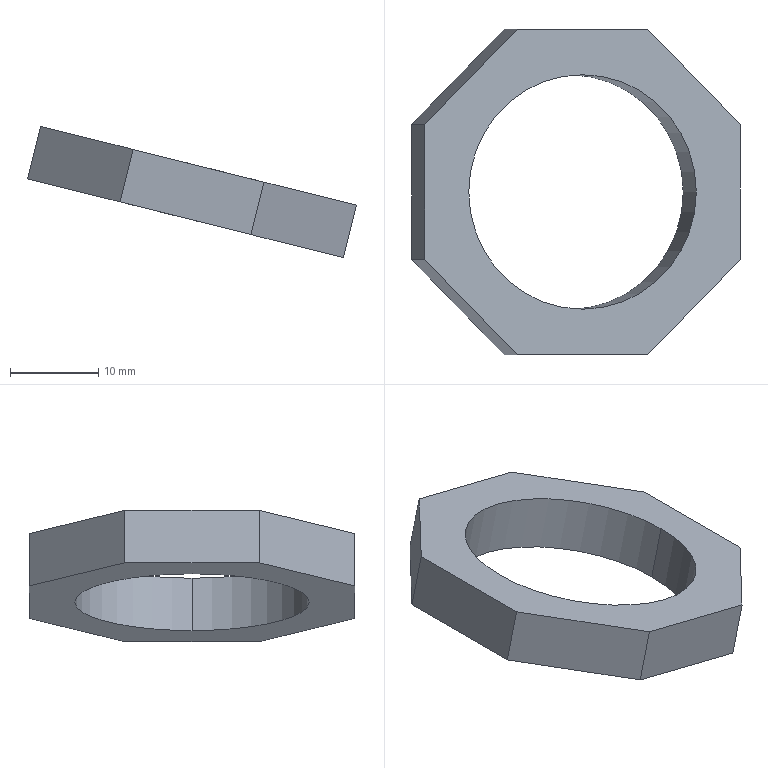Part | SolidWorks | features BaseBody 1 | 1 solid | 12 faces | box 37.183 x 36.8 x 14.82 mm | volume 3479 mm3 | plane 10 | cylinder 2 | commonest cylinder face diameters 26.5 x2
STEP:
#1=CARTESIAN_POINT('',(-437.833,-4.,307.747));
#2=VERTEX_POINT('',#1);
#3=CARTESIAN_POINT('',(-463.547,-4.,314.157));
#4=VERTEX_POINT('',#3);
#5=CARTESIAN_POINT('',(-450.69,-4.,310.952));
#6=DIRECTION('',(0.2419,0.,0.9703));
#7=DIRECTION('',(0.9703,0.,-0.2419));
#8=AXIS2_PLACEMENT_3D('',#5,#6,#7);
#9=CIRCLE('',#8,13.25);
#10=EDGE_CURVE('',#2,#4,#9,.T.);
#11=ORIENTED_EDGE('',*,*,#10,.F.);
#12=CARTESIAN_POINT('',(-436.358,-4.,313.666));
#13=VERTEX_POINT('',#12);
#14=CARTESIAN_POINT('',(-437.833,-4.,307.747));
#15=DIRECTION('',(0.2419,0.,0.9703));
#16=VECTOR('',#15,1000.);
#17=LINE('',#14,#16);
#18=EDGE_CURVE('',#2,#13,#17,.T.);
#19=ORIENTED_EDGE('',*,*,#18,.T.);
#20=CARTESIAN_POINT('',(-462.071,-4.,320.076));
#21=VERTEX_POINT('',#20);
#22=CARTESIAN_POINT('',(-449.215,-4.,316.871));
#23=DIRECTION('',(0.2419,0.,0.9703));
#24=DIRECTION('',(0.9703,0.,-0.2419));
#25=AXIS2_PLACEMENT_3D('',#22,#23,#24);
#26=CIRCLE('',#25,13.25);
#27=EDGE_CURVE('',#13,#21,#26,.T.);
#28=ORIENTED_EDGE('',*,*,#27,.T.);
#29=CARTESIAN_POINT('',(-463.547,-4.,314.157));
#30=DIRECTION('',(0.2419,0.,0.9703));
#31=VECTOR('',#30,1000.);
#32=LINE('',#29,#31);
#33=EDGE_CURVE('',#4,#21,#32,.T.);
#34=ORIENTED_EDGE('',*,*,#33,.F.);
#35=EDGE_LOOP('',(#11,#19,#28,#34));
#36=FACE_OUTER_BOUND('',#35,.T.);
#37=CARTESIAN_POINT('',(-450.69,-4.,310.952));
#38=DIRECTION('',(0.2419,0.,0.9703));
#39=DIRECTION('',(-0.9703,0.,0.2419));
#40=AXIS2_PLACEMENT_3D('',#37,#38,#39);
#41=CYLINDRICAL_SURFACE('',#40,13.25);
#42=ADVANCED_FACE('',(#36),#41,.F.);
#43=CARTESIAN_POINT('',(-449.215,-4.,316.871));
#44=DIRECTION('',(0.2419,0.,0.9703));
#45=DIRECTION('',(0.9703,0.,-0.2419));
#46=AXIS2_PLACEMENT_3D('',#43,#44,#45);
#47=CIRCLE('',#46,13.25);
#48=EDGE_CURVE('',#21,#13,#47,.T.);
#49=ORIENTED_EDGE('',*,*,#48,.F.);
#50=ORIENTED_EDGE('',*,*,#27,.F.);
#51=EDGE_LOOP('',(#49,#50));
#52=FACE_BOUND('',#51,.T.);
#53=CARTESIAN_POINT('',(-467.068,3.622,321.321));
#54=VERTEX_POINT('',#53);
#55=CARTESIAN_POINT('',(-467.068,-11.622,321.321));
#56=VERTEX_POINT('',#55);
#57=CARTESIAN_POINT('',(-467.068,-4.,321.321));
#58=DIRECTION('',(0.,-1.,0.));
#59=VECTOR('',#58,1000.);
#60=LINE('',#57,#59);
#61=EDGE_CURVE('',#54,#56,#60,.T.);
#62=ORIENTED_EDGE('',*,*,#61,.T.);
#63=CARTESIAN_POINT('',(-456.61,-22.4,318.714));
#64=VERTEX_POINT('',#63);
#65=CARTESIAN_POINT('',(-461.839,-17.011,320.018));
#66=DIRECTION('',(0.6861,-0.7071,-0.171));
#67=VECTOR('',#66,1000.);
#68=LINE('',#65,#67);
#69=EDGE_CURVE('',#56,#64,#68,.T.);
#70=ORIENTED_EDGE('',*,*,#69,.T.);
#71=CARTESIAN_POINT('',(-441.819,-22.4,315.027));
#72=VERTEX_POINT('',#71);
#73=CARTESIAN_POINT('',(-449.215,-22.4,316.871));
#74=DIRECTION('',(0.9703,0.,-0.2419));
#75=VECTOR('',#74,1000.);
#76=LINE('',#73,#75);
#77=EDGE_CURVE('',#64,#72,#76,.T.);
#78=ORIENTED_EDGE('',*,*,#77,.T.);
#79=CARTESIAN_POINT('',(-431.361,-11.622,312.42));
#80=VERTEX_POINT('',#79);
#81=CARTESIAN_POINT('',(-436.59,-17.011,313.724));
#82=DIRECTION('',(0.6861,0.7071,-0.171));
#83=VECTOR('',#82,1000.);
#84=LINE('',#81,#83);
#85=EDGE_CURVE('',#72,#80,#84,.T.);
#86=ORIENTED_EDGE('',*,*,#85,.T.);
#87=CARTESIAN_POINT('',(-431.361,3.622,312.42));
#88=VERTEX_POINT('',#87);
#89=CARTESIAN_POINT('',(-431.361,-4.,312.42));
#90=DIRECTION('',(0.,1.,0.));
#91=VECTOR('',#90,1000.);
#92=LINE('',#89,#91);
#93=EDGE_CURVE('',#80,#88,#92,.T.);
#94=ORIENTED_EDGE('',*,*,#93,.T.);
#95=CARTESIAN_POINT('',(-441.819,14.4,315.027));
#96=VERTEX_POINT('',#95);
#97=CARTESIAN_POINT('',(-436.59,9.011,313.724));
#98=DIRECTION('',(-0.6861,0.7071,0.171));
#99=VECTOR('',#98,1000.);
#100=LINE('',#97,#99);
#101=EDGE_CURVE('',#88,#96,#100,.T.);
#102=ORIENTED_EDGE('',*,*,#101,.T.);
#103=CARTESIAN_POINT('',(-456.61,14.4,318.714));
#104=VERTEX_POINT('',#103);
#105=CARTESIAN_POINT('',(-449.215,14.4,316.871));
#106=DIRECTION('',(-0.9703,0.,0.2419));
#107=VECTOR('',#106,1000.);
#108=LINE('',#105,#107);
#109=EDGE_CURVE('',#96,#104,#108,.T.);
#110=ORIENTED_EDGE('',*,*,#109,.T.);
#111=CARTESIAN_POINT('',(-461.839,9.011,320.018));
#112=DIRECTION('',(-0.6861,-0.7071,0.171));
#113=VECTOR('',#112,1000.);
#114=LINE('',#111,#113);
#115=EDGE_CURVE('',#104,#54,#114,.T.);
#116=ORIENTED_EDGE('',*,*,#115,.T.);
#117=EDGE_LOOP('',(#62,#70,#78,#86,#94,#102,#110,#116));
#118=FACE_OUTER_BOUND('',#117,.T.);
#119=CARTESIAN_POINT('',(-449.215,-4.,316.871));
#120=DIRECTION('',(0.2419,0.,0.9703));
#121=DIRECTION('',(0.,-1.,0.));
#122=AXIS2_PLACEMENT_3D('',#119,#120,#121);
#123=PLANE('',#122);
#124=ADVANCED_FACE('',(#52,#118),#123,.T.);
#125=CARTESIAN_POINT('',(-450.69,-4.,310.952));
#126=DIRECTION('',(0.2419,0.,0.9703));
#127=DIRECTION('',(0.9703,0.,-0.2419));
#128=AXIS2_PLACEMENT_3D('',#125,#126,#127);
#129=CIRCLE('',#128,13.25);
#130=EDGE_CURVE('',#4,#2,#129,.T.);
#131=ORIENTED_EDGE('',*,*,#130,.T.);
#132=ORIENTED_EDGE('',*,*,#10,.T.);
#133=EDGE_LOOP('',(#131,#132));
#134=FACE_BOUND('',#133,.T.);
#135=CARTESIAN_POINT('',(-468.544,3.622,315.403));
#136=VERTEX_POINT('',#135);
#137=CARTESIAN_POINT('',(-468.544,-11.622,315.403));
#138=VERTEX_POINT('',#137);
#139=CARTESIAN_POINT('',(-468.544,3.622,315.403));
#140=DIRECTION('',(0.,-1.,0.));
#141=VECTOR('',#140,1000.);
#142=LINE('',#139,#141);
#143=EDGE_CURVE('',#136,#138,#142,.T.);
#144=ORIENTED_EDGE('',*,*,#143,.F.);
#145=CARTESIAN_POINT('',(-458.085,14.4,312.795));
#146=VERTEX_POINT('',#145);
#147=CARTESIAN_POINT('',(-458.085,14.4,312.795));
#148=DIRECTION('',(-0.6861,-0.7071,0.171));
#149=VECTOR('',#148,1000.);
#150=LINE('',#147,#149);
#151=EDGE_CURVE('',#146,#136,#150,.T.);
#152=ORIENTED_EDGE('',*,*,#151,.F.);
#153=CARTESIAN_POINT('',(-443.295,14.4,309.108));
#154=VERTEX_POINT('',#153);
#155=CARTESIAN_POINT('',(-443.295,14.4,309.108));
#156=DIRECTION('',(-0.9703,0.,0.2419));
#157=VECTOR('',#156,1000.);
#158=LINE('',#155,#157);
#159=EDGE_CURVE('',#154,#146,#158,.T.);
#160=ORIENTED_EDGE('',*,*,#159,.F.);
#161=CARTESIAN_POINT('',(-432.836,3.622,306.501));
#162=VERTEX_POINT('',#161);
#163=CARTESIAN_POINT('',(-432.836,3.622,306.501));
#164=DIRECTION('',(-0.6861,0.7071,0.171));
#165=VECTOR('',#164,1000.);
#166=LINE('',#163,#165);
#167=EDGE_CURVE('',#162,#154,#166,.T.);
#168=ORIENTED_EDGE('',*,*,#167,.F.);
#169=CARTESIAN_POINT('',(-432.836,-11.622,306.501));
#170=VERTEX_POINT('',#169);
#171=CARTESIAN_POINT('',(-432.836,-11.622,306.501));
#172=DIRECTION('',(0.,1.,0.));
#173=VECTOR('',#172,1000.);
#174=LINE('',#171,#173);
#175=EDGE_CURVE('',#170,#162,#174,.T.);
#176=ORIENTED_EDGE('',*,*,#175,.F.);
#177=CARTESIAN_POINT('',(-443.295,-22.4,309.108));
#178=VERTEX_POINT('',#177);
#179=CARTESIAN_POINT('',(-443.295,-22.4,309.108));
#180=DIRECTION('',(0.6861,0.7071,-0.171));
#181=VECTOR('',#180,1000.);
#182=LINE('',#179,#181);
#183=EDGE_CURVE('',#178,#170,#182,.T.);
#184=ORIENTED_EDGE('',*,*,#183,.F.);
#185=CARTESIAN_POINT('',(-458.085,-22.4,312.795));
#186=VERTEX_POINT('',#185);
#187=CARTESIAN_POINT('',(-458.085,-22.4,312.795));
#188=DIRECTION('',(0.9703,0.,-0.2419));
#189=VECTOR('',#188,1000.);
#190=LINE('',#187,#189);
#191=EDGE_CURVE('',#186,#178,#190,.T.);
#192=ORIENTED_EDGE('',*,*,#191,.F.);
#193=CARTESIAN_POINT('',(-468.544,-11.622,315.403));
#194=DIRECTION('',(0.6861,-0.7071,-0.171));
#195=VECTOR('',#194,1000.);
#196=LINE('',#193,#195);
#197=EDGE_CURVE('',#138,#186,#196,.T.);
#198=ORIENTED_EDGE('',*,*,#197,.F.);
#199=EDGE_LOOP('',(#144,#152,#160,#168,#176,#184,#192,#198));
#200=FACE_OUTER_BOUND('',#199,.T.);
#201=CARTESIAN_POINT('',(-450.69,-4.,310.952));
#202=DIRECTION('',(0.2419,0.,0.9703));
#203=DIRECTION('',(0.,-1.,0.));
#204=AXIS2_PLACEMENT_3D('',#201,#202,#203);
#205=PLANE('',#204);
#206=ADVANCED_FACE('',(#134,#200),#205,.F.);
#207=ORIENTED_EDGE('',*,*,#115,.F.);
#208=CARTESIAN_POINT('',(-458.085,14.4,312.795));
#209=DIRECTION('',(0.2419,0.,0.9703));
#210=VECTOR('',#209,1000.);
#211=LINE('',#208,#210);
#212=EDGE_CURVE('',#146,#104,#211,.T.);
#213=ORIENTED_EDGE('',*,*,#212,.F.);
#214=ORIENTED_EDGE('',*,*,#151,.T.);
#215=CARTESIAN_POINT('',(-468.544,3.622,315.403));
#216=DIRECTION('',(0.2419,0.,0.9703));
#217=VECTOR('',#216,1000.);
#218=LINE('',#215,#217);
#219=EDGE_CURVE('',#136,#54,#218,.T.);
#220=ORIENTED_EDGE('',*,*,#219,.T.);
#221=EDGE_LOOP('',(#207,#213,#214,#220));
#222=FACE_OUTER_BOUND('',#221,.T.);
#223=CARTESIAN_POINT('',(-458.085,14.4,312.795));
#224=DIRECTION('',(-0.6861,0.7071,0.171));
#225=DIRECTION('',(0.2419,0.,0.9703));
#226=AXIS2_PLACEMENT_3D('',#223,#224,#225);
#227=PLANE('',#226);
#228=ADVANCED_FACE('',(#222),#227,.T.);
#229=ORIENTED_EDGE('',*,*,#109,.F.);
#230=CARTESIAN_POINT('',(-443.295,14.4,309.108));
#231=DIRECTION('',(0.2419,0.,0.9703));
#232=VECTOR('',#231,1000.);
#233=LINE('',#230,#232);
#234=EDGE_CURVE('',#154,#96,#233,.T.);
#235=ORIENTED_EDGE('',*,*,#234,.F.);
#236=ORIENTED_EDGE('',*,*,#159,.T.);
#237=ORIENTED_EDGE('',*,*,#212,.T.);
#238=EDGE_LOOP('',(#229,#235,#236,#237));
#239=FACE_OUTER_BOUND('',#238,.T.);
#240=CARTESIAN_POINT('',(-443.295,14.4,309.108));
#241=DIRECTION('',(0.,1.,0.));
#242=DIRECTION('',(1.,0.,0.));
#243=AXIS2_PLACEMENT_3D('',#240,#241,#242);
#244=PLANE('',#243);
#245=ADVANCED_FACE('',(#239),#244,.T.);
#246=ORIENTED_EDGE('',*,*,#101,.F.);
#247=CARTESIAN_POINT('',(-432.836,3.622,306.501));
#248=DIRECTION('',(0.2419,0.,0.9703));
#249=VECTOR('',#248,1000.);
#250=LINE('',#247,#249);
#251=EDGE_CURVE('',#162,#88,#250,.T.);
#252=ORIENTED_EDGE('',*,*,#251,.F.);
#253=ORIENTED_EDGE('',*,*,#167,.T.);
#254=ORIENTED_EDGE('',*,*,#234,.T.);
#255=EDGE_LOOP('',(#246,#252,#253,#254));
#256=FACE_OUTER_BOUND('',#255,.T.);
#257=CARTESIAN_POINT('',(-432.836,3.622,306.501));
#258=DIRECTION('',(0.6861,0.7071,-0.171));
#259=DIRECTION('',(-0.2419,0.,-0.9703));
#260=AXIS2_PLACEMENT_3D('',#257,#258,#259);
#261=PLANE('',#260);
#262=ADVANCED_FACE('',(#256),#261,.T.);
#263=ORIENTED_EDGE('',*,*,#93,.F.);
#264=CARTESIAN_POINT('',(-432.836,-11.622,306.501));
#265=DIRECTION('',(0.2419,0.,0.9703));
#266=VECTOR('',#265,1000.);
#267=LINE('',#264,#266);
#268=EDGE_CURVE('',#170,#80,#267,.T.);
#269=ORIENTED_EDGE('',*,*,#268,.F.);
#270=ORIENTED_EDGE('',*,*,#175,.T.);
#271=ORIENTED_EDGE('',*,*,#251,.T.);
#272=EDGE_LOOP('',(#263,#269,#270,#271));
#273=FACE_OUTER_BOUND('',#272,.T.);
#274=CARTESIAN_POINT('',(-432.836,-11.622,306.501));
#275=DIRECTION('',(0.9703,0.,-0.2419));
#276=DIRECTION('',(0.,-1.,0.));
#277=AXIS2_PLACEMENT_3D('',#274,#275,#276);
#278=PLANE('',#277);
#279=ADVANCED_FACE('',(#273),#278,.T.);
#280=ORIENTED_EDGE('',*,*,#85,.F.);
#281=CARTESIAN_POINT('',(-443.295,-22.4,309.108));
#282=DIRECTION('',(0.2419,0.,0.9703));
#283=VECTOR('',#282,1000.);
#284=LINE('',#281,#283);
#285=EDGE_CURVE('',#178,#72,#284,.T.);
#286=ORIENTED_EDGE('',*,*,#285,.F.);
#287=ORIENTED_EDGE('',*,*,#183,.T.);
#288=ORIENTED_EDGE('',*,*,#268,.T.);
#289=EDGE_LOOP('',(#280,#286,#287,#288));
#290=FACE_OUTER_BOUND('',#289,.T.);
#291=CARTESIAN_POINT('',(-443.295,-22.4,309.108));
#292=DIRECTION('',(0.6861,-0.7071,-0.171));
#293=DIRECTION('',(0.,0.2351,-0.972));
#294=AXIS2_PLACEMENT_3D('',#291,#292,#293);
#295=PLANE('',#294);
#296=ADVANCED_FACE('',(#290),#295,.T.);
#297=ORIENTED_EDGE('',*,*,#77,.F.);
#298=CARTESIAN_POINT('',(-458.085,-22.4,312.795));
#299=DIRECTION('',(0.2419,0.,0.9703));
#300=VECTOR('',#299,1000.);
#301=LINE('',#298,#300);
#302=EDGE_CURVE('',#186,#64,#301,.T.);
#303=ORIENTED_EDGE('',*,*,#302,.F.);
#304=ORIENTED_EDGE('',*,*,#191,.T.);
#305=ORIENTED_EDGE('',*,*,#285,.T.);
#306=EDGE_LOOP('',(#297,#303,#304,#305));
#307=FACE_OUTER_BOUND('',#306,.T.);
#308=CARTESIAN_POINT('',(-458.085,-22.4,312.795));
#309=DIRECTION('',(0.,-1.,0.));
#310=DIRECTION('',(-1.,0.,0.));
#311=AXIS2_PLACEMENT_3D('',#308,#309,#310);
#312=PLANE('',#311);
#313=ADVANCED_FACE('',(#307),#312,.T.);
#314=ORIENTED_EDGE('',*,*,#69,.F.);
#315=CARTESIAN_POINT('',(-468.544,-11.622,315.403));
#316=DIRECTION('',(0.2419,0.,0.9703));
#317=VECTOR('',#316,1000.);
#318=LINE('',#315,#317);
#319=EDGE_CURVE('',#138,#56,#318,.T.);
#320=ORIENTED_EDGE('',*,*,#319,.F.);
#321=ORIENTED_EDGE('',*,*,#197,.T.);
#322=ORIENTED_EDGE('',*,*,#302,.T.);
#323=EDGE_LOOP('',(#314,#320,#321,#322));
#324=FACE_OUTER_BOUND('',#323,.T.);
#325=CARTESIAN_POINT('',(-468.544,-11.622,315.403));
#326=DIRECTION('',(-0.6861,-0.7071,0.171));
#327=DIRECTION('',(-0.7177,0.6964,0.));
#328=AXIS2_PLACEMENT_3D('',#325,#326,#327);
#329=PLANE('',#328);
#330=ADVANCED_FACE('',(#324),#329,.T.);
#331=ORIENTED_EDGE('',*,*,#61,.F.);
#332=ORIENTED_EDGE('',*,*,#219,.F.);
#333=ORIENTED_EDGE('',*,*,#143,.T.);
#334=ORIENTED_EDGE('',*,*,#319,.T.);
#335=EDGE_LOOP('',(#331,#332,#333,#334));
#336=FACE_OUTER_BOUND('',#335,.T.);
#337=CARTESIAN_POINT('',(-468.544,3.622,315.403));
#338=DIRECTION('',(-0.9703,0.,0.2419));
#339=DIRECTION('',(0.,1.,0.));
#340=AXIS2_PLACEMENT_3D('',#337,#338,#339);
#341=PLANE('',#340);
#342=ADVANCED_FACE('',(#336),#341,.T.);
#343=ORIENTED_EDGE('',*,*,#18,.F.);
#344=ORIENTED_EDGE('',*,*,#130,.F.);
#345=ORIENTED_EDGE('',*,*,#33,.T.);
#346=ORIENTED_EDGE('',*,*,#48,.T.);
#347=EDGE_LOOP('',(#343,#344,#345,#346));
#348=FACE_OUTER_BOUND('',#347,.T.);
#349=CARTESIAN_POINT('',(-450.69,-4.,310.952));
#350=DIRECTION('',(0.2419,0.,0.9703));
#351=DIRECTION('',(-0.9703,0.,0.2419));
#352=AXIS2_PLACEMENT_3D('',#349,#350,#351);
#353=CYLINDRICAL_SURFACE('',#352,13.25);
#354=ADVANCED_FACE('',(#348),#353,.F.);
#355=CLOSED_SHELL('',(#42,#124,#206,#228,#245,#262,#279,#296,#313,#330,#342,#354));
#356=MANIFOLD_SOLID_BREP('',#355);
#357=CARTESIAN_POINT('',(0.,0.,0.));
#358=DIRECTION('',(0.,0.,1.));
#359=DIRECTION('',(1.,0.,0.));
#360=AXIS2_PLACEMENT_3D('',#357,#358,#359);
#361=(LENGTH_UNIT()NAMED_UNIT(*)SI_UNIT(.MILLI.,.METRE.));
#362=UNCERTAINTY_MEASURE_WITH_UNIT(LENGTH_MEASURE(0.00001),#361,'','');
#363=(NAMED_UNIT(*)PLANE_ANGLE_UNIT()SI_UNIT($,.RADIAN.));
#364=(NAMED_UNIT(*)SI_UNIT($,.STERADIAN.)SOLID_ANGLE_UNIT());
#365=(GEOMETRIC_REPRESENTATION_CONTEXT(3)GLOBAL_UNCERTAINTY_ASSIGNED_CONTEXT((#362))GLOBAL_UNIT_ASSIGNED_CONTEXT((#361,#363,#364))REPRESENTATION_CONTEXT('',''));
#366=ADVANCED_BREP_SHAPE_REPRESENTATION('',(#356,#360),#365);